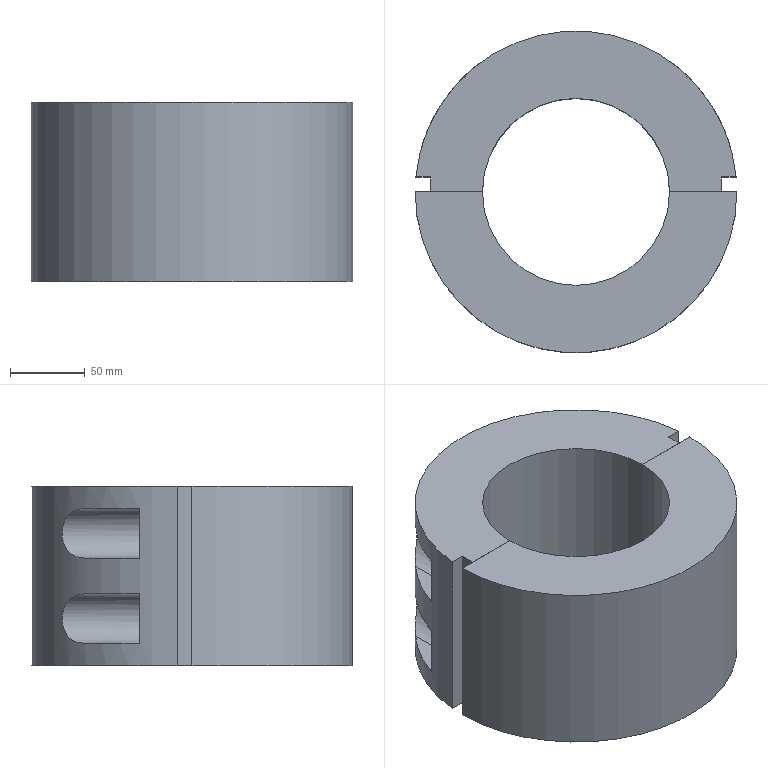NC program | NX | posted with a generic post | part box 215 x 215 x 120 mm
Lines 5811 to 5839 of 5839:
(DRILLING , TOOL : ZXZ)
N11620 T02 M6
N11622 G54
N11624 G17 G0 G90 X80. Y-28.5 S3500 M3
N11626 G43 Z30. H2
N11628 G94 G81 G98 Z-73.5 F250. R-69.5
N11630 Y28.5
N11632 X-80.
N11634 Y-28.5
N11636 G80
N11638 G0 X-80. Y-28.5 Z30.
N11640 M5
(DRILLING_COPY , TOOL : 21.5ZT)
N11642 T03 M6
N11644 G54
N11646 G17 G0 G90 X-80. Y28.5 S500 M3
N11648 G43 Z30. H3
N11650 G94 G83 G98 Z-115.459 F80. Q3. R-69.5
N11652 Y-28.5
N11654 X80.
N11656 Y28.5
N11658 G80
N11660 G0 X80. Y28.5 Z30.
N11662 M5
N11664 M2